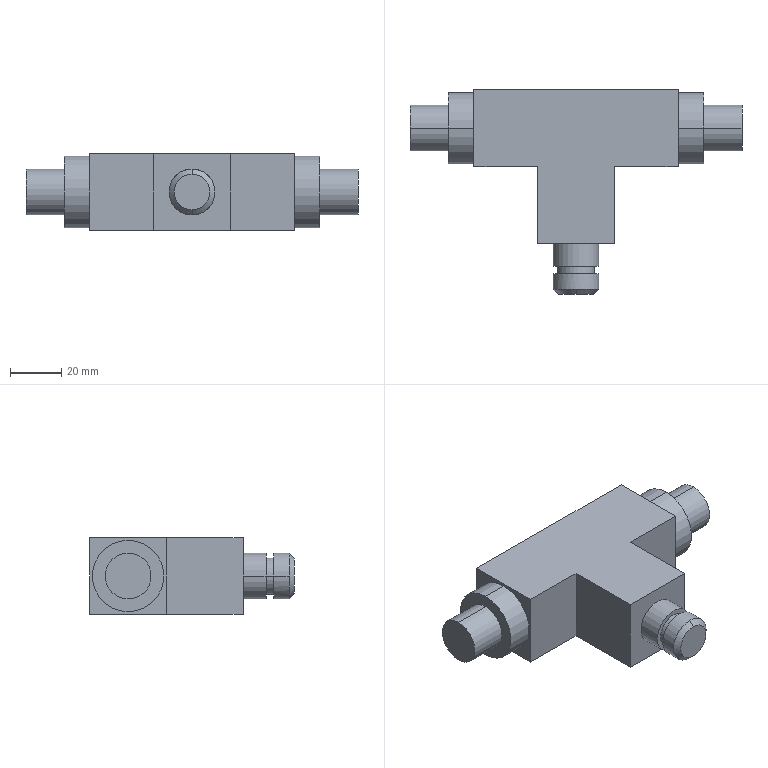Part | SolidWorks | features ICE 6, Chamfer 1, Cut 1, Extrusion 1 | 1 solid | 39 faces | box 130 x 80 x 30 mm | volume 123416 mm3 | plane 19 | cylinder 18 | cone 2 | commonest cylinder face diameters 18 x8 5 x4 28 x4 14.296 x2
STEP:
#1=CARTESIAN_POINT('',(-17.5,45.,6.));
#2=VERTEX_POINT('',#1);
#3=CARTESIAN_POINT('',(-22.5,45.,6.));
#4=VERTEX_POINT('',#3);
#5=CARTESIAN_POINT('',(-20.,45.,6.));
#6=DIRECTION('',(0.,0.,-1.));
#7=DIRECTION('',(-1.,0.,0.));
#8=AXIS2_PLACEMENT_3D('',#5,#6,#7);
#9=CIRCLE('',#8,2.5);
#10=EDGE_CURVE('',#2,#4,#9,.T.);
#11=ORIENTED_EDGE('',*,*,#10,.F.);
#12=CARTESIAN_POINT('',(-17.5,45.,0.));
#13=VERTEX_POINT('',#12);
#14=CARTESIAN_POINT('',(-17.5,45.,6.));
#15=DIRECTION('',(0.,0.,-1.));
#16=VECTOR('',#15,1000.);
#17=LINE('',#14,#16);
#18=EDGE_CURVE('',#2,#13,#17,.T.);
#19=ORIENTED_EDGE('',*,*,#18,.T.);
#20=CARTESIAN_POINT('',(-22.5,45.,0.));
#21=VERTEX_POINT('',#20);
#22=CARTESIAN_POINT('',(-20.,45.,0.));
#23=DIRECTION('',(0.,0.,-1.));
#24=DIRECTION('',(-1.,0.,0.));
#25=AXIS2_PLACEMENT_3D('',#22,#23,#24);
#26=CIRCLE('',#25,2.5);
#27=EDGE_CURVE('',#13,#21,#26,.T.);
#28=ORIENTED_EDGE('',*,*,#27,.T.);
#29=CARTESIAN_POINT('',(-22.5,45.,6.));
#30=DIRECTION('',(0.,0.,-1.));
#31=VECTOR('',#30,1000.);
#32=LINE('',#29,#31);
#33=EDGE_CURVE('',#4,#21,#32,.T.);
#34=ORIENTED_EDGE('',*,*,#33,.F.);
#35=EDGE_LOOP('',(#11,#19,#28,#34));
#36=FACE_OUTER_BOUND('',#35,.T.);
#37=CARTESIAN_POINT('',(-20.,45.,6.));
#38=DIRECTION('',(0.,0.,-1.));
#39=DIRECTION('',(-1.,0.,0.));
#40=AXIS2_PLACEMENT_3D('',#37,#38,#39);
#41=CYLINDRICAL_SURFACE('',#40,2.5);
#42=ADVANCED_FACE('',(#36),#41,.F.);
#43=CARTESIAN_POINT('',(52.5,45.,6.));
#44=VERTEX_POINT('',#43);
#45=CARTESIAN_POINT('',(47.5,45.,6.));
#46=VERTEX_POINT('',#45);
#47=CARTESIAN_POINT('',(50.,45.,6.));
#48=DIRECTION('',(0.,0.,-1.));
#49=DIRECTION('',(-1.,0.,0.));
#50=AXIS2_PLACEMENT_3D('',#47,#48,#49);
#51=CIRCLE('',#50,2.5);
#52=EDGE_CURVE('',#44,#46,#51,.T.);
#53=ORIENTED_EDGE('',*,*,#52,.F.);
#54=CARTESIAN_POINT('',(52.5,45.,0.));
#55=VERTEX_POINT('',#54);
#56=CARTESIAN_POINT('',(52.5,45.,6.));
#57=DIRECTION('',(0.,0.,-1.));
#58=VECTOR('',#57,1000.);
#59=LINE('',#56,#58);
#60=EDGE_CURVE('',#44,#55,#59,.T.);
#61=ORIENTED_EDGE('',*,*,#60,.T.);
#62=CARTESIAN_POINT('',(47.5,45.,0.));
#63=VERTEX_POINT('',#62);
#64=CARTESIAN_POINT('',(50.,45.,0.));
#65=DIRECTION('',(0.,0.,-1.));
#66=DIRECTION('',(-1.,0.,0.));
#67=AXIS2_PLACEMENT_3D('',#64,#65,#66);
#68=CIRCLE('',#67,2.5);
#69=EDGE_CURVE('',#55,#63,#68,.T.);
#70=ORIENTED_EDGE('',*,*,#69,.T.);
#71=CARTESIAN_POINT('',(47.5,45.,6.));
#72=DIRECTION('',(0.,0.,-1.));
#73=VECTOR('',#72,1000.);
#74=LINE('',#71,#73);
#75=EDGE_CURVE('',#46,#63,#74,.T.);
#76=ORIENTED_EDGE('',*,*,#75,.F.);
#77=EDGE_LOOP('',(#53,#61,#70,#76));
#78=FACE_OUTER_BOUND('',#77,.T.);
#79=CARTESIAN_POINT('',(50.,45.,6.));
#80=DIRECTION('',(0.,0.,-1.));
#81=DIRECTION('',(-1.,0.,0.));
#82=AXIS2_PLACEMENT_3D('',#79,#80,#81);
#83=CYLINDRICAL_SURFACE('',#82,2.5);
#84=ADVANCED_FACE('',(#78),#83,.F.);
#85=CARTESIAN_POINT('',(15.,-20.,8.));
#86=VERTEX_POINT('',#85);
#87=CARTESIAN_POINT('',(15.,-20.,22.));
#88=VERTEX_POINT('',#87);
#89=CARTESIAN_POINT('',(15.,-20.,15.));
#90=DIRECTION('',(0.,-1.,0.));
#91=DIRECTION('',(1.,0.,0.));
#92=AXIS2_PLACEMENT_3D('',#89,#90,#91);
#93=CIRCLE('',#92,7.);
#94=EDGE_CURVE('',#86,#88,#93,.T.);
#95=ORIENTED_EDGE('',*,*,#94,.F.);
#96=CARTESIAN_POINT('',(15.,-18.,6.));
#97=VERTEX_POINT('',#96);
#98=CARTESIAN_POINT('',(15.,-20.,8.));
#99=DIRECTION('',(0.,0.7071,-0.7071));
#100=VECTOR('',#99,1000.);
#101=LINE('',#98,#100);
#102=EDGE_CURVE('',#86,#97,#101,.T.);
#103=ORIENTED_EDGE('',*,*,#102,.T.);
#104=CARTESIAN_POINT('',(24.,-18.,15.));
#105=VERTEX_POINT('',#104);
#106=CARTESIAN_POINT('',(15.,-18.,15.));
#107=DIRECTION('',(0.,1.,0.));
#108=DIRECTION('',(0.,0.,-1.));
#109=AXIS2_PLACEMENT_3D('',#106,#107,#108);
#110=CIRCLE('',#109,9.);
#111=EDGE_CURVE('',#105,#97,#110,.T.);
#112=ORIENTED_EDGE('',*,*,#111,.F.);
#113=CARTESIAN_POINT('',(15.,-18.,24.));
#114=VERTEX_POINT('',#113);
#115=CARTESIAN_POINT('',(15.,-18.,15.));
#116=DIRECTION('',(0.,1.,0.));
#117=DIRECTION('',(0.,0.,-1.));
#118=AXIS2_PLACEMENT_3D('',#115,#116,#117);
#119=CIRCLE('',#118,9.);
#120=EDGE_CURVE('',#114,#105,#119,.T.);
#121=ORIENTED_EDGE('',*,*,#120,.F.);
#122=CARTESIAN_POINT('',(15.,-20.,22.));
#123=DIRECTION('',(0.,0.7071,0.7071));
#124=VECTOR('',#123,1000.);
#125=LINE('',#122,#124);
#126=EDGE_CURVE('',#88,#114,#125,.T.);
#127=ORIENTED_EDGE('',*,*,#126,.F.);
#128=EDGE_LOOP('',(#95,#103,#112,#121,#127));
#129=FACE_OUTER_BOUND('',#128,.T.);
#130=CARTESIAN_POINT('',(15.,-20.,15.));
#131=DIRECTION('',(0.,1.,0.));
#132=DIRECTION('',(0.,0.,1.));
#133=AXIS2_PLACEMENT_3D('',#130,#131,#132);
#134=CONICAL_SURFACE('',#133,7.,0.7854);
#135=ADVANCED_FACE('',(#129),#134,.T.);
#136=CARTESIAN_POINT('',(6.,-18.,15.));
#137=VERTEX_POINT('',#136);
#138=CARTESIAN_POINT('',(15.,-18.,15.));
#139=DIRECTION('',(0.,1.,0.));
#140=DIRECTION('',(0.,0.,-1.));
#141=AXIS2_PLACEMENT_3D('',#138,#139,#140);
#142=CIRCLE('',#141,9.);
#143=EDGE_CURVE('',#137,#114,#142,.T.);
#144=ORIENTED_EDGE('',*,*,#143,.T.);
#145=ORIENTED_EDGE('',*,*,#120,.T.);
#146=CARTESIAN_POINT('',(24.,-12.,15.));
#147=VERTEX_POINT('',#146);
#148=CARTESIAN_POINT('',(24.,-20.,15.));
#149=DIRECTION('',(0.,1.,0.));
#150=VECTOR('',#149,1000.);
#151=LINE('',#148,#150);
#152=EDGE_CURVE('',#105,#147,#151,.T.);
#153=ORIENTED_EDGE('',*,*,#152,.T.);
#154=CARTESIAN_POINT('',(6.,-12.,15.));
#155=VERTEX_POINT('',#154);
#156=CARTESIAN_POINT('',(15.,-12.,15.));
#157=DIRECTION('',(0.,-1.,0.));
#158=DIRECTION('',(1.,0.,0.));
#159=AXIS2_PLACEMENT_3D('',#156,#157,#158);
#160=CIRCLE('',#159,9.);
#161=EDGE_CURVE('',#147,#155,#160,.T.);
#162=ORIENTED_EDGE('',*,*,#161,.T.);
#163=CARTESIAN_POINT('',(6.,-20.,15.));
#164=DIRECTION('',(0.,1.,0.));
#165=VECTOR('',#164,1000.);
#166=LINE('',#163,#165);
#167=EDGE_CURVE('',#137,#155,#166,.T.);
#168=ORIENTED_EDGE('',*,*,#167,.F.);
#169=EDGE_LOOP('',(#144,#145,#153,#162,#168));
#170=FACE_OUTER_BOUND('',#169,.T.);
#171=CARTESIAN_POINT('',(15.,-20.,15.));
#172=DIRECTION('',(0.,1.,0.));
#173=DIRECTION('',(-1.,0.,0.));
#174=AXIS2_PLACEMENT_3D('',#171,#172,#173);
#175=CYLINDRICAL_SURFACE('',#174,9.);
#176=ADVANCED_FACE('',(#170),#175,.T.);
#177=CARTESIAN_POINT('',(22.148,-9.,15.));
#178=VERTEX_POINT('',#177);
#179=CARTESIAN_POINT('',(7.852,-9.,15.));
#180=VERTEX_POINT('',#179);
#181=CARTESIAN_POINT('',(15.,-9.,15.));
#182=DIRECTION('',(0.,-1.,0.));
#183=DIRECTION('',(1.,0.,0.));
#184=AXIS2_PLACEMENT_3D('',#181,#182,#183);
#185=CIRCLE('',#184,7.148);
#186=EDGE_CURVE('',#178,#180,#185,.T.);
#187=ORIENTED_EDGE('',*,*,#186,.T.);
#188=CARTESIAN_POINT('',(7.852,-12.,15.));
#189=VERTEX_POINT('',#188);
#190=CARTESIAN_POINT('',(7.852,-9.,15.));
#191=DIRECTION('',(0.,-1.,0.));
#192=VECTOR('',#191,1000.);
#193=LINE('',#190,#192);
#194=EDGE_CURVE('',#180,#189,#193,.T.);
#195=ORIENTED_EDGE('',*,*,#194,.T.);
#196=CARTESIAN_POINT('',(22.148,-12.,15.));
#197=VERTEX_POINT('',#196);
#198=CARTESIAN_POINT('',(15.,-12.,15.));
#199=DIRECTION('',(0.,-1.,0.));
#200=DIRECTION('',(1.,0.,0.));
#201=AXIS2_PLACEMENT_3D('',#198,#199,#200);
#202=CIRCLE('',#201,7.148);
#203=EDGE_CURVE('',#197,#189,#202,.T.);
#204=ORIENTED_EDGE('',*,*,#203,.F.);
#205=CARTESIAN_POINT('',(22.148,-9.,15.));
#206=DIRECTION('',(0.,-1.,0.));
#207=VECTOR('',#206,1000.);
#208=LINE('',#205,#207);
#209=EDGE_CURVE('',#178,#197,#208,.T.);
#210=ORIENTED_EDGE('',*,*,#209,.F.);
#211=EDGE_LOOP('',(#187,#195,#204,#210));
#212=FACE_OUTER_BOUND('',#211,.T.);
#213=CARTESIAN_POINT('',(15.,-9.,15.));
#214=DIRECTION('',(0.,-1.,0.));
#215=DIRECTION('',(1.,0.,0.));
#216=AXIS2_PLACEMENT_3D('',#213,#214,#215);
#217=CYLINDRICAL_SURFACE('',#216,7.148);
#218=ADVANCED_FACE('',(#212),#217,.T.);
#219=CARTESIAN_POINT('',(-50.,45.,24.));
#220=VERTEX_POINT('',#219);
#221=CARTESIAN_POINT('',(-50.,45.,6.));
#222=VERTEX_POINT('',#221);
#223=CARTESIAN_POINT('',(-50.,45.,15.));
#224=DIRECTION('',(-1.,0.,0.));
#225=DIRECTION('',(0.,0.,1.));
#226=AXIS2_PLACEMENT_3D('',#223,#224,#225);
#227=CIRCLE('',#226,9.);
#228=EDGE_CURVE('',#220,#222,#227,.T.);
#229=ORIENTED_EDGE('',*,*,#228,.F.);
#230=CARTESIAN_POINT('',(-35.,45.,24.));
#231=VERTEX_POINT('',#230);
#232=CARTESIAN_POINT('',(-50.,45.,24.));
#233=DIRECTION('',(1.,0.,0.));
#234=VECTOR('',#233,1000.);
#235=LINE('',#232,#234);
#236=EDGE_CURVE('',#220,#231,#235,.T.);
#237=ORIENTED_EDGE('',*,*,#236,.T.);
#238=CARTESIAN_POINT('',(-35.,45.,6.));
#239=VERTEX_POINT('',#238);
#240=CARTESIAN_POINT('',(-35.,45.,15.));
#241=DIRECTION('',(-1.,0.,0.));
#242=DIRECTION('',(0.,0.,1.));
#243=AXIS2_PLACEMENT_3D('',#240,#241,#242);
#244=CIRCLE('',#243,9.);
#245=EDGE_CURVE('',#231,#239,#244,.T.);
#246=ORIENTED_EDGE('',*,*,#245,.T.);
#247=CARTESIAN_POINT('',(-50.,45.,6.));
#248=DIRECTION('',(1.,0.,0.));
#249=VECTOR('',#248,1000.);
#250=LINE('',#247,#249);
#251=EDGE_CURVE('',#222,#239,#250,.T.);
#252=ORIENTED_EDGE('',*,*,#251,.F.);
#253=EDGE_LOOP('',(#229,#237,#246,#252));
#254=FACE_OUTER_BOUND('',#253,.T.);
#255=CARTESIAN_POINT('',(-50.,45.,15.));
#256=DIRECTION('',(1.,0.,0.));
#257=DIRECTION('',(0.,0.,-1.));
#258=AXIS2_PLACEMENT_3D('',#255,#256,#257);
#259=CYLINDRICAL_SURFACE('',#258,9.);
#260=ADVANCED_FACE('',(#254),#259,.T.);
#261=CARTESIAN_POINT('',(-35.,45.,29.));
#262=VERTEX_POINT('',#261);
#263=CARTESIAN_POINT('',(-35.,45.,1.));
#264=VERTEX_POINT('',#263);
#265=CARTESIAN_POINT('',(-35.,45.,15.));
#266=DIRECTION('',(-1.,0.,0.));
#267=DIRECTION('',(0.,0.,1.));
#268=AXIS2_PLACEMENT_3D('',#265,#266,#267);
#269=CIRCLE('',#268,14.);
#270=EDGE_CURVE('',#262,#264,#269,.T.);
#271=ORIENTED_EDGE('',*,*,#270,.F.);
#272=CARTESIAN_POINT('',(-25.,45.,29.));
#273=VERTEX_POINT('',#272);
#274=CARTESIAN_POINT('',(-35.,45.,29.));
#275=DIRECTION('',(1.,0.,0.));
#276=VECTOR('',#275,1000.);
#277=LINE('',#274,#276);
#278=EDGE_CURVE('',#262,#273,#277,.T.);
#279=ORIENTED_EDGE('',*,*,#278,.T.);
#280=CARTESIAN_POINT('',(-25.,45.,1.));
#281=VERTEX_POINT('',#280);
#282=CARTESIAN_POINT('',(-25.,45.,15.));
#283=DIRECTION('',(-1.,0.,0.));
#284=DIRECTION('',(0.,0.,-1.));
#285=AXIS2_PLACEMENT_3D('',#282,#283,#284);
#286=CIRCLE('',#285,14.);
#287=EDGE_CURVE('',#273,#281,#286,.T.);
#288=ORIENTED_EDGE('',*,*,#287,.T.);
#289=CARTESIAN_POINT('',(-35.,45.,1.));
#290=DIRECTION('',(1.,0.,0.));
#291=VECTOR('',#290,1000.);
#292=LINE('',#289,#291);
#293=EDGE_CURVE('',#264,#281,#292,.T.);
#294=ORIENTED_EDGE('',*,*,#293,.F.);
#295=EDGE_LOOP('',(#271,#279,#288,#294));
#296=FACE_OUTER_BOUND('',#295,.T.);
#297=CARTESIAN_POINT('',(-35.,45.,15.));
#298=DIRECTION('',(1.,0.,0.));
#299=DIRECTION('',(0.,0.,-1.));
#300=AXIS2_PLACEMENT_3D('',#297,#298,#299);
#301=CYLINDRICAL_SURFACE('',#300,14.);
#302=ADVANCED_FACE('',(#296),#301,.T.);
#303=CARTESIAN_POINT('',(80.,45.,6.));
#304=VERTEX_POINT('',#303);
#305=CARTESIAN_POINT('',(80.,45.,24.));
#306=VERTEX_POINT('',#305);
#307=CARTESIAN_POINT('',(80.,45.,15.));
#308=DIRECTION('',(1.,0.,0.));
#309=DIRECTION('',(0.,0.,-1.));
#310=AXIS2_PLACEMENT_3D('',#307,#308,#309);
#311=CIRCLE('',#310,9.);
#312=EDGE_CURVE('',#304,#306,#311,.T.);
#313=ORIENTED_EDGE('',*,*,#312,.F.);
#314=CARTESIAN_POINT('',(65.,45.,6.));
#315=VERTEX_POINT('',#314);
#316=CARTESIAN_POINT('',(80.,45.,6.));
#317=DIRECTION('',(-1.,0.,0.));
#318=VECTOR('',#317,1000.);
#319=LINE('',#316,#318);
#320=EDGE_CURVE('',#304,#315,#319,.T.);
#321=ORIENTED_EDGE('',*,*,#320,.T.);
#322=CARTESIAN_POINT('',(65.,45.,24.));
#323=VERTEX_POINT('',#322);
#324=CARTESIAN_POINT('',(65.,45.,15.));
#325=DIRECTION('',(1.,0.,0.));
#326=DIRECTION('',(0.,0.,-1.));
#327=AXIS2_PLACEMENT_3D('',#324,#325,#326);
#328=CIRCLE('',#327,9.);
#329=EDGE_CURVE('',#315,#323,#328,.T.);
#330=ORIENTED_EDGE('',*,*,#329,.T.);
#331=CARTESIAN_POINT('',(80.,45.,24.));
#332=DIRECTION('',(-1.,0.,0.));
#333=VECTOR('',#332,1000.);
#334=LINE('',#331,#333);
#335=EDGE_CURVE('',#306,#323,#334,.T.);
#336=ORIENTED_EDGE('',*,*,#335,.F.);
#337=EDGE_LOOP('',(#313,#321,#330,#336));
#338=FACE_OUTER_BOUND('',#337,.T.);
#339=CARTESIAN_POINT('',(80.,45.,15.));
#340=DIRECTION('',(-1.,0.,0.));
#341=DIRECTION('',(0.,0.,1.));
#342=AXIS2_PLACEMENT_3D('',#339,#340,#341);
#343=CYLINDRICAL_SURFACE('',#342,9.);
#344=ADVANCED_FACE('',(#338),#343,.T.);
#345=CARTESIAN_POINT('',(65.,45.,1.));
#346=VERTEX_POINT('',#345);
#347=CARTESIAN_POINT('',(65.,45.,29.));
#348=VERTEX_POINT('',#347);
#349=CARTESIAN_POINT('',(65.,45.,15.));
#350=DIRECTION('',(1.,0.,0.));
#351=DIRECTION('',(0.,0.,-1.));
#352=AXIS2_PLACEMENT_3D('',#349,#350,#351);
#353=CIRCLE('',#352,14.);
#354=EDGE_CURVE('',#346,#348,#353,.T.);
#355=ORIENTED_EDGE('',*,*,#354,.F.);
#356=CARTESIAN_POINT('',(55.,45.,1.));
#357=VERTEX_POINT('',#356);
#358=CARTESIAN_POINT('',(65.,45.,1.));
#359=DIRECTION('',(-1.,0.,0.));
#360=VECTOR('',#359,1000.);
#361=LINE('',#358,#360);
#362=EDGE_CURVE('',#346,#357,#361,.T.);
#363=ORIENTED_EDGE('',*,*,#362,.T.);
#364=CARTESIAN_POINT('',(55.,45.,29.));
#365=VERTEX_POINT('',#364);
#366=CARTESIAN_POINT('',(55.,45.,15.));
#367=DIRECTION('',(1.,0.,0.));
#368=DIRECTION('',(0.,-1.,0.));
#369=AXIS2_PLACEMENT_3D('',#366,#367,#368);
#370=CIRCLE('',#369,14.);
#371=EDGE_CURVE('',#357,#365,#370,.T.);
#372=ORIENTED_EDGE('',*,*,#371,.T.);
#373=CARTESIAN_POINT('',(65.,45.,29.));
#374=DIRECTION('',(-1.,0.,0.));
#375=VECTOR('',#374,1000.);
#376=LINE('',#373,#375);
#377=EDGE_CURVE('',#348,#365,#376,.T.);
#378=ORIENTED_EDGE('',*,*,#377,.F.);
#379=EDGE_LOOP('',(#355,#363,#372,#378));
#380=FACE_OUTER_BOUND('',#379,.T.);
#381=CARTESIAN_POINT('',(65.,45.,15.));
#382=DIRECTION('',(-1.,0.,0.));
#383=DIRECTION('',(0.,0.,1.));
#384=AXIS2_PLACEMENT_3D('',#381,#382,#383);
#385=CYLINDRICAL_SURFACE('',#384,14.);
#386=ADVANCED_FACE('',(#380),#385,.T.);
#387=CARTESIAN_POINT('',(24.,-9.,15.));
#388=VERTEX_POINT('',#387);
#389=CARTESIAN_POINT('',(6.,-9.,15.));
#390=VERTEX_POINT('',#389);
#391=CARTESIAN_POINT('',(15.,-9.,15.));
#392=DIRECTION('',(0.,-1.,0.));
#393=DIRECTION('',(1.,0.,0.));
#394=AXIS2_PLACEMENT_3D('',#391,#392,#393);
#395=CIRCLE('',#394,9.);
#396=EDGE_CURVE('',#388,#390,#395,.T.);
#397=ORIENTED_EDGE('',*,*,#396,.F.);
#398=CARTESIAN_POINT('',(24.,0.,15.));
#399=VERTEX_POINT('',#398);
#400=CARTESIAN_POINT('',(24.,-20.,15.));
#401=DIRECTION('',(0.,1.,0.));
#402=VECTOR('',#401,1000.);
#403=LINE('',#400,#402);
#404=EDGE_CURVE('',#388,#399,#403,.T.);
#405=ORIENTED_EDGE('',*,*,#404,.T.);
#406=CARTESIAN_POINT('',(6.,0.,15.));
#407=VERTEX_POINT('',#406);
#408=CARTESIAN_POINT('',(15.,0.,15.));
#409=DIRECTION('',(0.,-1.,0.));
#410=DIRECTION('',(-1.,0.,0.));
#411=AXIS2_PLACEMENT_3D('',#408,#409,#410);
#412=CIRCLE('',#411,9.);
#413=EDGE_CURVE('',#399,#407,#412,.T.);
#414=ORIENTED_EDGE('',*,*,#413,.T.);
#415=CARTESIAN_POINT('',(6.,-20.,15.));
#416=DIRECTION('',(0.,1.,0.));
#417=VECTOR('',#416,1000.);
#418=LINE('',#415,#417);
#419=EDGE_CURVE('',#390,#407,#418,.T.);
#420=ORIENTED_EDGE('',*,*,#419,.F.);
#421=EDGE_LOOP('',(#397,#405,#414,#420));
#422=FACE_OUTER_BOUND('',#421,.T.);
#423=CARTESIAN_POINT('',(15.,-20.,15.));
#424=DIRECTION('',(0.,1.,0.));
#425=DIRECTION('',(-1.,0.,0.));
#426=AXIS2_PLACEMENT_3D('',#423,#424,#425);
#427=CYLINDRICAL_SURFACE('',#426,9.);
#428=ADVANCED_FACE('',(#422),#427,.T.);
#429=ORIENTED_EDGE('',*,*,#404,.F.);
#430=CARTESIAN_POINT('',(15.,-9.,15.));
#431=DIRECTION('',(0.,-1.,0.));
#432=DIRECTION('',(1.,0.,0.));
#433=AXIS2_PLACEMENT_3D('',#430,#431,#432);
#434=CIRCLE('',#433,9.);
#435=EDGE_CURVE('',#390,#388,#434,.T.);
#436=ORIENTED_EDGE('',*,*,#435,.F.);
#437=ORIENTED_EDGE('',*,*,#419,.T.);
#438=CARTESIAN_POINT('',(15.,0.,15.));
#439=DIRECTION('',(0.,-1.,0.));
#440=DIRECTION('',(-1.,0.,0.));
#441=AXIS2_PLACEMENT_3D('',#438,#439,#440);
#442=CIRCLE('',#441,9.);
#443=EDGE_CURVE('',#407,#399,#442,.T.);
#444=ORIENTED_EDGE('',*,*,#443,.T.);
#445=EDGE_LOOP('',(#429,#436,#437,#444));
#446=FACE_OUTER_BOUND('',#445,.T.);
#447=CARTESIAN_POINT('',(15.,-20.,15.));
#448=DIRECTION('',(0.,1.,0.));
#449=DIRECTION('',(-1.,0.,0.));
#450=AXIS2_PLACEMENT_3D('',#447,#448,#449);
#451=CYLINDRICAL_SURFACE('',#450,9.);
#452=ADVANCED_FACE('',(#446),#451,.T.);
#453=ORIENTED_EDGE('',*,*,#443,.F.);
#454=ORIENTED_EDGE('',*,*,#413,.F.);
#455=EDGE_LOOP('',(#453,#454));
#456=FACE_BOUND('',#455,.T.);
#457=CARTESIAN_POINT('',(0.,0.,0.));
#458=VERTEX_POINT('',#457);
#459=CARTESIAN_POINT('',(30.,0.,0.));
#460=VERTEX_POINT('',#459);
#461=CARTESIAN_POINT('',(30.,0.,0.));
#462=DIRECTION('',(1.,0.,0.));
#463=VECTOR('',#462,1000.);
#464=LINE('',#461,#463);
#465=EDGE_CURVE('',#458,#460,#464,.T.);
#466=ORIENTED_EDGE('',*,*,#465,.T.);
#467=CARTESIAN_POINT('',(30.,0.,30.));
#468=VERTEX_POINT('',#467);
#469=CARTESIAN_POINT('',(30.,0.,30.));
#470=DIRECTION('',(0.,0.,-1.));
#471=VECTOR('',#470,1000.);
#472=LINE('',#469,#471);
#473=EDGE_CURVE('',#468,#460,#472,.T.);
#474=ORIENTED_EDGE('',*,*,#473,.F.);
#475=CARTESIAN_POINT('',(0.,0.,30.));
#476=VERTEX_POINT('',#475);
#477=CARTESIAN_POINT('',(30.,0.,30.));
#478=DIRECTION('',(1.,0.,0.));
#479=VECTOR('',#478,1000.);
#480=LINE('',#477,#479);
#481=EDGE_CURVE('',#476,#468,#480,.T.);
#482=ORIENTED_EDGE('',*,*,#481,.F.);
#483=CARTESIAN_POINT('',(0.,0.,30.));
#484=DIRECTION('',(0.,0.,-1.));
#485=VECTOR('',#484,1000.);
#486=LINE('',#483,#485);
#487=EDGE_CURVE('',#476,#458,#486,.T.);
#488=ORIENTED_EDGE('',*,*,#487,.T.);
#489=EDGE_LOOP('',(#466,#474,#482,#488));
#490=FACE_OUTER_BOUND('',#489,.T.);
#491=CARTESIAN_POINT('',(30.,0.,30.));
#492=DIRECTION('',(0.,1.,0.));
#493=DIRECTION('',(-1.,0.,0.));
#494=AXIS2_PLACEMENT_3D('',#491,#492,#493);
#495=PLANE('',#494);
#496=ADVANCED_FACE('',(#456,#490),#495,.F.);
#497=CARTESIAN_POINT('',(30.,30.,0.));
#498=VERTEX_POINT('',#497);
#499=CARTESIAN_POINT('',(30.,30.,0.));
#500=DIRECTION('',(0.,1.,0.));
#501=VECTOR('',#500,1000.);
#502=LINE('',#499,#501);
#503=EDGE_CURVE('',#460,#498,#502,.T.);
#504=ORIENTED_EDGE('',*,*,#503,.T.);
#505=CARTESIAN_POINT('',(30.,30.,30.));
#506=VERTEX_POINT('',#505);
#507=CARTESIAN_POINT('',(30.,30.,30.));
#508=DIRECTION('',(0.,0.,-1.));
#509=VECTOR('',#508,1000.);
#510=LINE('',#507,#509);
#511=EDGE_CURVE('',#506,#498,#510,.T.);
#512=ORIENTED_EDGE('',*,*,#511,.F.);
#513=CARTESIAN_POINT('',(30.,30.,30.));
#514=DIRECTION('',(0.,1.,0.));
#515=VECTOR('',#514,1000.);
#516=LINE('',#513,#515);
#517=EDGE_CURVE('',#468,#506,#516,.T.);
#518=ORIENTED_EDGE('',*,*,#517,.F.);
#519=ORIENTED_EDGE('',*,*,#473,.T.);
#520=EDGE_LOOP('',(#504,#512,#518,#519));
#521=FACE_OUTER_BOUND('',#520,.T.);
#522=CARTESIAN_POINT('',(30.,30.,30.));
#523=DIRECTION('',(-1.,0.,0.));
#524=DIRECTION('',(0.,-1.,0.));
#525=AXIS2_PLACEMENT_3D('',#522,#523,#524);
#526=PLANE('',#525);
#527=ADVANCED_FACE('',(#521),#526,.F.);
#528=CARTESIAN_POINT('',(55.,30.,0.));
#529=VERTEX_POINT('',#528);
#530=CARTESIAN_POINT('',(55.,30.,0.));
#531=DIRECTION('',(1.,0.,0.));
#532=VECTOR('',#531,1000.);
#533=LINE('',#530,#532);
#534=EDGE_CURVE('',#498,#529,#533,.T.);
#535=ORIENTED_EDGE('',*,*,#534,.T.);
#536=CARTESIAN_POINT('',(55.,30.,30.));
#537=VERTEX_POINT('',#536);
#538=CARTESIAN_POINT('',(55.,30.,30.));
#539=DIRECTION('',(0.,0.,-1.));
#540=VECTOR('',#539,1000.);
#541=LINE('',#538,#540);
#542=EDGE_CURVE('',#537,#529,#541,.T.);
#543=ORIENTED_EDGE('',*,*,#542,.F.);
#544=CARTESIAN_POINT('',(55.,30.,30.));
#545=DIRECTION('',(1.,0.,0.));
#546=VECTOR('',#545,1000.);
#547=LINE('',#544,#546);
#548=EDGE_CURVE('',#506,#537,#547,.T.);
#549=ORIENTED_EDGE('',*,*,#548,.F.);
#550=ORIENTED_EDGE('',*,*,#511,.T.);
#551=EDGE_LOOP('',(#535,#543,#549,#550));
#552=FACE_OUTER_BOUND('',#551,.T.);
#553=CARTESIAN_POINT('',(55.,30.,30.));
#554=DIRECTION('',(0.,1.,0.));
#555=DIRECTION('',(0.,0.,1.));
#556=AXIS2_PLACEMENT_3D('',#553,#554,#555);
#557=PLANE('',#556);
#558=ADVANCED_FACE('',(#552),#557,.F.);
#559=CARTESIAN_POINT('',(55.,45.,15.));
#560=DIRECTION('',(1.,0.,0.));
#561=DIRECTION('',(0.,-1.,0.));
#562=AXIS2_PLACEMENT_3D('',#559,#560,#561);
#563=CIRCLE('',#562,14.);
#564=EDGE_CURVE('',#365,#357,#563,.T.);
#565=ORIENTED_EDGE('',*,*,#564,.F.);
#566=ORIENTED_EDGE('',*,*,#371,.F.);
#567=EDGE_LOOP('',(#565,#566));
#568=FACE_BOUND('',#567,.T.);
#569=CARTESIAN_POINT('',(55.,60.,0.));
#570=VERTEX_POINT('',#569);
#571=CARTESIAN_POINT('',(55.,60.,0.));
#572=DIRECTION('',(0.,1.,0.));
#573=VECTOR('',#572,1000.);
#574=LINE('',#571,#573);
#575=EDGE_CURVE('',#529,#570,#574,.T.);
#576=ORIENTED_EDGE('',*,*,#575,.T.);
#577=CARTESIAN_POINT('',(55.,60.,30.));
#578=VERTEX_POINT('',#577);
#579=CARTESIAN_POINT('',(55.,60.,30.));
#580=DIRECTION('',(0.,0.,-1.));
#581=VECTOR('',#580,1000.);
#582=LINE('',#579,#581);
#583=EDGE_CURVE('',#578,#570,#582,.T.);
#584=ORIENTED_EDGE('',*,*,#583,.F.);
#585=CARTESIAN_POINT('',(55.,60.,30.));
#586=DIRECTION('',(0.,1.,0.));
#587=VECTOR('',#586,1000.);
#588=LINE('',#585,#587);
#589=EDGE_CURVE('',#537,#578,#588,.T.);
#590=ORIENTED_EDGE('',*,*,#589,.F.);
#591=ORIENTED_EDGE('',*,*,#542,.T.);
#592=EDGE_LOOP('',(#576,#584,#590,#591));
#593=FACE_OUTER_BOUND('',#592,.T.);
#594=CARTESIAN_POINT('',(55.,60.,30.));
#595=DIRECTION('',(-1.,0.,0.));
#596=DIRECTION('',(0.,-1.,0.));
#597=AXIS2_PLACEMENT_3D('',#594,#595,#596);
#598=PLANE('',#597);
#599=ADVANCED_FACE('',(#568,#593),#598,.F.);
#600=CARTESIAN_POINT('',(-25.,60.,0.));
#601=VERTEX_POINT('',#600);
#602=CARTESIAN_POINT('',(-25.,60.,0.));
#603=DIRECTION('',(-1.,0.,0.));
#604=VECTOR('',#603,1000.);
#605=LINE('',#602,#604);
#606=EDGE_CURVE('',#570,#601,#605,.T.);
#607=ORIENTED_EDGE('',*,*,#606,.T.);
#608=CARTESIAN_POINT('',(-25.,60.,30.));
#609=VERTEX_POINT('',#608);
#610=CARTESIAN_POINT('',(-25.,60.,30.));
#611=DIRECTION('',(0.,0.,-1.));
#612=VECTOR('',#611,1000.);
#613=LINE('',#610,#612);
#614=EDGE_CURVE('',#609,#601,#613,.T.);
#615=ORIENTED_EDGE('',*,*,#614,.F.);
#616=CARTESIAN_POINT('',(-25.,60.,30.));
#617=DIRECTION('',(-1.,0.,0.));
#618=VECTOR('',#617,1000.);
#619=LINE('',#616,#618);
#620=EDGE_CURVE('',#578,#609,#619,.T.);
#621=ORIENTED_EDGE('',*,*,#620,.F.);
#622=ORIENTED_EDGE('',*,*,#583,.T.);
#623=EDGE_LOOP('',(#607,#615,#621,#622));
#624=FACE_OUTER_BOUND('',#623,.T.);
#625=CARTESIAN_POINT('',(-25.,60.,30.));
#626=DIRECTION('',(0.,-1.,0.));
#627=DIRECTION('',(1.,0.,0.));
#628=AXIS2_PLACEMENT_3D('',#625,#626,#627);
#629=PLANE('',#628);
#630=ADVANCED_FACE('',(#624),#629,.F.);
#631=CARTESIAN_POINT('',(-25.,45.,15.));
#632=DIRECTION('',(-1.,0.,0.));
#633=DIRECTION('',(0.,0.,-1.));
#634=AXIS2_PLACEMENT_3D('',#631,#632,#633);
#635=CIRCLE('',#634,14.);
#636=EDGE_CURVE('',#281,#273,#635,.T.);
#637=ORIENTED_EDGE('',*,*,#636,.F.);
#638=ORIENTED_EDGE('',*,*,#287,.F.);
#639=EDGE_LOOP('',(#637,#638));
#640=FACE_BOUND('',#639,.T.);
#641=CARTESIAN_POINT('',(-25.,30.,0.));
#642=VERTEX_POINT('',#641);
#643=CARTESIAN_POINT('',(-25.,30.,0.));
#644=DIRECTION('',(0.,-1.,0.));
#645=VECTOR('',#644,1000.);
#646=LINE('',#643,#645);
#647=EDGE_CURVE('',#601,#642,#646,.T.);
#648=ORIENTED_EDGE('',*,*,#647,.T.);
#649=CARTESIAN_POINT('',(-25.,30.,30.));
#650=VERTEX_POINT('',#649);
#651=CARTESIAN_POINT('',(-25.,30.,30.));
#652=DIRECTION('',(0.,0.,-1.));
#653=VECTOR('',#652,1000.);
#654=LINE('',#651,#653);
#655=EDGE_CURVE('',#650,#642,#654,.T.);
#656=ORIENTED_EDGE('',*,*,#655,.F.);
#657=CARTESIAN_POINT('',(-25.,30.,30.));
#658=DIRECTION('',(0.,-1.,0.));
#659=VECTOR('',#658,1000.);
#660=LINE('',#657,#659);
#661=EDGE_CURVE('',#609,#650,#660,.T.);
#662=ORIENTED_EDGE('',*,*,#661,.F.);
#663=ORIENTED_EDGE('',*,*,#614,.T.);
#664=EDGE_LOOP('',(#648,#656,#662,#663));
#665=FACE_OUTER_BOUND('',#664,.T.);
#666=CARTESIAN_POINT('',(-25.,30.,30.));
#667=DIRECTION('',(1.,0.,0.));
#668=DIRECTION('',(0.,0.,-1.));
#669=AXIS2_PLACEMENT_3D('',#666,#667,#668);
#670=PLANE('',#669);
#671=ADVANCED_FACE('',(#640,#665),#670,.F.);
#672=CARTESIAN_POINT('',(0.,30.,0.));
#673=VERTEX_POINT('',#672);
#674=CARTESIAN_POINT('',(0.,30.,0.));
#675=DIRECTION('',(1.,0.,0.));
#676=VECTOR('',#675,1000.);
#677=LINE('',#674,#676);
#678=EDGE_CURVE('',#642,#673,#677,.T.);
#679=ORIENTED_EDGE('',*,*,#678,.T.);
#680=CARTESIAN_POINT('',(0.,30.,30.));
#681=VERTEX_POINT('',#680);
#682=CARTESIAN_POINT('',(0.,30.,30.));
#683=DIRECTION('',(0.,0.,-1.));
#684=VECTOR('',#683,1000.);
#685=LINE('',#682,#684);
#686=EDGE_CURVE('',#681,#673,#685,.T.);
#687=ORIENTED_EDGE('',*,*,#686,.F.);
#688=CARTESIAN_POINT('',(0.,30.,30.));
#689=DIRECTION('',(1.,0.,0.));
#690=VECTOR('',#689,1000.);
#691=LINE('',#688,#690);
#692=EDGE_CURVE('',#650,#681,#691,.T.);
#693=ORIENTED_EDGE('',*,*,#692,.F.);
#694=ORIENTED_EDGE('',*,*,#655,.T.);
#695=EDGE_LOOP('',(#679,#687,#693,#694));
#696=FACE_OUTER_BOUND('',#695,.T.);
#697=CARTESIAN_POINT('',(0.,30.,30.));
#698=DIRECTION('',(0.,1.,0.));
#699=DIRECTION('',(-1.,0.,0.));
#700=AXIS2_PLACEMENT_3D('',#697,#698,#699);
#701=PLANE('',#700);
#702=ADVANCED_FACE('',(#696),#701,.F.);
#703=CARTESIAN_POINT('',(0.,0.,0.));
#704=DIRECTION('',(0.,-1.,0.));
#705=VECTOR('',#704,1000.);
#706=LINE('',#703,#705);
#707=EDGE_CURVE('',#673,#458,#706,.T.);
#708=ORIENTED_EDGE('',*,*,#707,.T.);
#709=ORIENTED_EDGE('',*,*,#487,.F.);
#710=CARTESIAN_POINT('',(0.,0.,30.));
#711=DIRECTION('',(0.,-1.,0.));
#712=VECTOR('',#711,1000.);
#713=LINE('',#710,#712);
#714=EDGE_CURVE('',#681,#476,#713,.T.);
#715=ORIENTED_EDGE('',*,*,#714,.F.);
#716=ORIENTED_EDGE('',*,*,#686,.T.);
#717=EDGE_LOOP('',(#708,#709,#715,#716));
#718=FACE_OUTER_BOUND('',#717,.T.);
#719=CARTESIAN_POINT('',(0.,0.,30.));
#720=DIRECTION('',(1.,0.,0.));
#721=DIRECTION('',(0.,0.,-1.));
#722=AXIS2_PLACEMENT_3D('',#719,#720,#721);
#723=PLANE('',#722);
#724=ADVANCED_FACE('',(#718),#723,.F.);
#725=ORIENTED_EDGE('',*,*,#481,.T.);
#726=ORIENTED_EDGE('',*,*,#517,.T.);
#727=ORIENTED_EDGE('',*,*,#548,.T.);
#728=ORIENTED_EDGE('',*,*,#589,.T.);
#729=ORIENTED_EDGE('',*,*,#620,.T.);
#730=ORIENTED_EDGE('',*,*,#661,.T.);
#731=ORIENTED_EDGE('',*,*,#692,.T.);
#732=ORIENTED_EDGE('',*,*,#714,.T.);
#733=EDGE_LOOP('',(#725,#726,#727,#728,#729,#730,#731,#732));
#734=FACE_OUTER_BOUND('',#733,.T.);
#735=CARTESIAN_POINT('',(0.,0.,30.));
#736=DIRECTION('',(0.,0.,-1.));
#737=DIRECTION('',(-1.,0.,0.));
#738=AXIS2_PLACEMENT_3D('',#735,#736,#737);
#739=PLANE('',#738);
#740=ADVANCED_FACE('',(#734),#739,.F.);
#741=CARTESIAN_POINT('',(-20.,45.,0.));
#742=DIRECTION('',(0.,0.,-1.));
#743=DIRECTION('',(-1.,0.,0.));
#744=AXIS2_PLACEMENT_3D('',#741,#742,#743);
#745=CIRCLE('',#744,2.5);
#746=EDGE_CURVE('',#21,#13,#745,.T.);
#747=ORIENTED_EDGE('',*,*,#746,.F.);
#748=ORIENTED_EDGE('',*,*,#27,.F.);
#749=EDGE_LOOP('',(#747,#748));
#750=FACE_BOUND('',#749,.T.);
#751=CARTESIAN_POINT('',(50.,45.,0.));
#752=DIRECTION('',(0.,0.,-1.));
#753=DIRECTION('',(-1.,0.,0.));
#754=AXIS2_PLACEMENT_3D('',#751,#752,#753);
#755=CIRCLE('',#754,2.5);
#756=EDGE_CURVE('',#63,#55,#755,.T.);
#757=ORIENTED_EDGE('',*,*,#756,.F.);
#758=ORIENTED_EDGE('',*,*,#69,.F.);
#759=EDGE_LOOP('',(#757,#758));
#760=FACE_BOUND('',#759,.T.);
#761=ORIENTED_EDGE('',*,*,#465,.F.);
#762=ORIENTED_EDGE('',*,*,#707,.F.);
#763=ORIENTED_EDGE('',*,*,#678,.F.);
#764=ORIENTED_EDGE('',*,*,#647,.F.);
#765=ORIENTED_EDGE('',*,*,#606,.F.);
#766=ORIENTED_EDGE('',*,*,#575,.F.);
#767=ORIENTED_EDGE('',*,*,#534,.F.);
#768=ORIENTED_EDGE('',*,*,#503,.F.);
#769=EDGE_LOOP('',(#761,#762,#763,#764,#765,#766,#767,#768));
#770=FACE_OUTER_BOUND('',#769,.T.);
#771=CARTESIAN_POINT('',(0.,0.,0.));
#772=DIRECTION('',(0.,0.,-1.));
#773=DIRECTION('',(-1.,0.,0.));
#774=AXIS2_PLACEMENT_3D('',#771,#772,#773);
#775=PLANE('',#774);
#776=ADVANCED_FACE('',(#750,#760,#770),#775,.T.);
#777=ORIENTED_EDGE('',*,*,#362,.F.);
#778=CARTESIAN_POINT('',(65.,45.,15.));
#779=DIRECTION('',(1.,0.,0.));
#780=DIRECTION('',(0.,0.,-1.));
#781=AXIS2_PLACEMENT_3D('',#778,#779,#780);
#782=CIRCLE('',#781,14.);
#783=EDGE_CURVE('',#348,#346,#782,.T.);
#784=ORIENTED_EDGE('',*,*,#783,.F.);
#785=ORIENTED_EDGE('',*,*,#377,.T.);
#786=ORIENTED_EDGE('',*,*,#564,.T.);
#787=EDGE_LOOP('',(#777,#784,#785,#786));
#788=FACE_OUTER_BOUND('',#787,.T.);
#789=CARTESIAN_POINT('',(65.,45.,15.));
#790=DIRECTION('',(-1.,0.,0.));
#791=DIRECTION('',(0.,0.,1.));
#792=AXIS2_PLACEMENT_3D('',#789,#790,#791);
#793=CYLINDRICAL_SURFACE('',#792,14.);
#794=ADVANCED_FACE('',(#788),#793,.T.);
#795=CARTESIAN_POINT('',(65.,45.,15.));
#796=DIRECTION('',(1.,0.,0.));
#797=DIRECTION('',(0.,0.,-1.));
#798=AXIS2_PLACEMENT_3D('',#795,#796,#797);
#799=CIRCLE('',#798,9.);
#800=EDGE_CURVE('',#323,#315,#799,.T.);
#801=ORIENTED_EDGE('',*,*,#800,.F.);
#802=ORIENTED_EDGE('',*,*,#329,.F.);
#803=EDGE_LOOP('',(#801,#802));
#804=FACE_BOUND('',#803,.T.);
#805=ORIENTED_EDGE('',*,*,#783,.T.);
#806=ORIENTED_EDGE('',*,*,#354,.T.);
#807=EDGE_LOOP('',(#805,#806));
#808=FACE_OUTER_BOUND('',#807,.T.);
#809=CARTESIAN_POINT('',(65.,45.,15.));
#810=DIRECTION('',(1.,0.,0.));
#811=DIRECTION('',(0.,0.,-1.));
#812=AXIS2_PLACEMENT_3D('',#809,#810,#811);
#813=PLANE('',#812);
#814=ADVANCED_FACE('',(#804,#808),#813,.T.);
#815=ORIENTED_EDGE('',*,*,#320,.F.);
#816=CARTESIAN_POINT('',(80.,45.,15.));
#817=DIRECTION('',(1.,0.,0.));
#818=DIRECTION('',(0.,0.,-1.));
#819=AXIS2_PLACEMENT_3D('',#816,#817,#818);
#820=CIRCLE('',#819,9.);
#821=EDGE_CURVE('',#306,#304,#820,.T.);
#822=ORIENTED_EDGE('',*,*,#821,.F.);
#823=ORIENTED_EDGE('',*,*,#335,.T.);
#824=ORIENTED_EDGE('',*,*,#800,.T.);
#825=EDGE_LOOP('',(#815,#822,#823,#824));
#826=FACE_OUTER_BOUND('',#825,.T.);
#827=CARTESIAN_POINT('',(80.,45.,15.));
#828=DIRECTION('',(-1.,0.,0.));
#829=DIRECTION('',(0.,0.,1.));
#830=AXIS2_PLACEMENT_3D('',#827,#828,#829);
#831=CYLINDRICAL_SURFACE('',#830,9.);
#832=ADVANCED_FACE('',(#826),#831,.T.);
#833=ORIENTED_EDGE('',*,*,#821,.T.);
#834=ORIENTED_EDGE('',*,*,#312,.T.);
#835=EDGE_LOOP('',(#833,#834));
#836=FACE_OUTER_BOUND('',#835,.T.);
#837=CARTESIAN_POINT('',(80.,45.,15.));
#838=DIRECTION('',(1.,0.,0.));
#839=DIRECTION('',(0.,0.,-1.));
#840=AXIS2_PLACEMENT_3D('',#837,#838,#839);
#841=PLANE('',#840);
#842=ADVANCED_FACE('',(#836),#841,.T.);
#843=ORIENTED_EDGE('',*,*,#278,.F.);
#844=CARTESIAN_POINT('',(-35.,45.,15.));
#845=DIRECTION('',(-1.,0.,0.));
#846=DIRECTION('',(0.,0.,1.));
#847=AXIS2_PLACEMENT_3D('',#844,#845,#846);
#848=CIRCLE('',#847,14.);
#849=EDGE_CURVE('',#264,#262,#848,.T.);
#850=ORIENTED_EDGE('',*,*,#849,.F.);
#851=ORIENTED_EDGE('',*,*,#293,.T.);
#852=ORIENTED_EDGE('',*,*,#636,.T.);
#853=EDGE_LOOP('',(#843,#850,#851,#852));
#854=FACE_OUTER_BOUND('',#853,.T.);
#855=CARTESIAN_POINT('',(-35.,45.,15.));
#856=DIRECTION('',(1.,0.,0.));
#857=DIRECTION('',(0.,0.,-1.));
#858=AXIS2_PLACEMENT_3D('',#855,#856,#857);
#859=CYLINDRICAL_SURFACE('',#858,14.);
#860=ADVANCED_FACE('',(#854),#859,.T.);
#861=CARTESIAN_POINT('',(-35.,45.,15.));
#862=DIRECTION('',(-1.,0.,0.));
#863=DIRECTION('',(0.,0.,1.));
#864=AXIS2_PLACEMENT_3D('',#861,#862,#863);
#865=CIRCLE('',#864,9.);
#866=EDGE_CURVE('',#239,#231,#865,.T.);
#867=ORIENTED_EDGE('',*,*,#866,.F.);
#868=ORIENTED_EDGE('',*,*,#245,.F.);
#869=EDGE_LOOP('',(#867,#868));
#870=FACE_BOUND('',#869,.T.);
#871=ORIENTED_EDGE('',*,*,#849,.T.);
#872=ORIENTED_EDGE('',*,*,#270,.T.);
#873=EDGE_LOOP('',(#871,#872));
#874=FACE_OUTER_BOUND('',#873,.T.);
#875=CARTESIAN_POINT('',(-35.,45.,15.));
#876=DIRECTION('',(-1.,0.,0.));
#877=DIRECTION('',(0.,0.,1.));
#878=AXIS2_PLACEMENT_3D('',#875,#876,#877);
#879=PLANE('',#878);
#880=ADVANCED_FACE('',(#870,#874),#879,.T.);
#881=ORIENTED_EDGE('',*,*,#236,.F.);
#882=CARTESIAN_POINT('',(-50.,45.,15.));
#883=DIRECTION('',(-1.,0.,0.));
#884=DIRECTION('',(0.,0.,1.));
#885=AXIS2_PLACEMENT_3D('',#882,#883,#884);
#886=CIRCLE('',#885,9.);
#887=EDGE_CURVE('',#222,#220,#886,.T.);
#888=ORIENTED_EDGE('',*,*,#887,.F.);
#889=ORIENTED_EDGE('',*,*,#251,.T.);
#890=ORIENTED_EDGE('',*,*,#866,.T.);
#891=EDGE_LOOP('',(#881,#888,#889,#890));
#892=FACE_OUTER_BOUND('',#891,.T.);
#893=CARTESIAN_POINT('',(-50.,45.,15.));
#894=DIRECTION('',(1.,0.,0.));
#895=DIRECTION('',(0.,0.,-1.));
#896=AXIS2_PLACEMENT_3D('',#893,#894,#895);
#897=CYLINDRICAL_SURFACE('',#896,9.);
#898=ADVANCED_FACE('',(#892),#897,.T.);
#899=ORIENTED_EDGE('',*,*,#887,.T.);
#900=ORIENTED_EDGE('',*,*,#228,.T.);
#901=EDGE_LOOP('',(#899,#900));
#902=FACE_OUTER_BOUND('',#901,.T.);
#903=CARTESIAN_POINT('',(-50.,45.,15.));
#904=DIRECTION('',(-1.,0.,0.));
#905=DIRECTION('',(0.,0.,1.));
#906=AXIS2_PLACEMENT_3D('',#903,#904,#905);
#907=PLANE('',#906);
#908=ADVANCED_FACE('',(#902),#907,.T.);
#909=ORIENTED_EDGE('',*,*,#186,.F.);
#910=CARTESIAN_POINT('',(15.,-9.,15.));
#911=DIRECTION('',(0.,-1.,0.));
#912=DIRECTION('',(1.,0.,0.));
#913=AXIS2_PLACEMENT_3D('',#910,#911,#912);
#914=CIRCLE('',#913,7.148);
#915=EDGE_CURVE('',#180,#178,#914,.T.);
#916=ORIENTED_EDGE('',*,*,#915,.F.);
#917=EDGE_LOOP('',(#909,#916));
#918=FACE_BOUND('',#917,.T.);
#919=ORIENTED_EDGE('',*,*,#435,.T.);
#920=ORIENTED_EDGE('',*,*,#396,.T.);
#921=EDGE_LOOP('',(#919,#920));
#922=FACE_OUTER_BOUND('',#921,.T.);
#923=CARTESIAN_POINT('',(15.,-9.,15.));
#924=DIRECTION('',(0.,-1.,0.));
#925=DIRECTION('',(1.,0.,0.));
#926=AXIS2_PLACEMENT_3D('',#923,#924,#925);
#927=PLANE('',#926);
#928=ADVANCED_FACE('',(#918,#922),#927,.T.);
#929=ORIENTED_EDGE('',*,*,#203,.T.);
#930=CARTESIAN_POINT('',(15.,-12.,15.));
#931=DIRECTION('',(0.,-1.,0.));
#932=DIRECTION('',(1.,0.,0.));
#933=AXIS2_PLACEMENT_3D('',#930,#931,#932);
#934=CIRCLE('',#933,7.148);
#935=EDGE_CURVE('',#189,#197,#934,.T.);
#936=ORIENTED_EDGE('',*,*,#935,.T.);
#937=EDGE_LOOP('',(#929,#936));
#938=FACE_BOUND('',#937,.T.);
#939=CARTESIAN_POINT('',(15.,-12.,15.));
#940=DIRECTION('',(0.,-1.,0.));
#941=DIRECTION('',(1.,0.,0.));
#942=AXIS2_PLACEMENT_3D('',#939,#940,#941);
#943=CIRCLE('',#942,9.);
#944=EDGE_CURVE('',#155,#147,#943,.T.);
#945=ORIENTED_EDGE('',*,*,#944,.F.);
#946=ORIENTED_EDGE('',*,*,#161,.F.);
#947=EDGE_LOOP('',(#945,#946));
#948=FACE_OUTER_BOUND('',#947,.T.);
#949=CARTESIAN_POINT('',(15.,-12.,15.));
#950=DIRECTION('',(0.,-1.,0.));
#951=DIRECTION('',(1.,0.,0.));
#952=AXIS2_PLACEMENT_3D('',#949,#950,#951);
#953=PLANE('',#952);
#954=ADVANCED_FACE('',(#938,#948),#953,.F.);
#955=ORIENTED_EDGE('',*,*,#194,.F.);
#956=ORIENTED_EDGE('',*,*,#915,.T.);
#957=ORIENTED_EDGE('',*,*,#209,.T.);
#958=ORIENTED_EDGE('',*,*,#935,.F.);
#959=EDGE_LOOP('',(#955,#956,#957,#958));
#960=FACE_OUTER_BOUND('',#959,.T.);
#961=CARTESIAN_POINT('',(15.,-9.,15.));
#962=DIRECTION('',(0.,-1.,0.));
#963=DIRECTION('',(1.,0.,0.));
#964=AXIS2_PLACEMENT_3D('',#961,#962,#963);
#965=CYLINDRICAL_SURFACE('',#964,7.148);
#966=ADVANCED_FACE('',(#960),#965,.T.);
#967=CARTESIAN_POINT('',(15.,-20.,15.));
#968=DIRECTION('',(0.,-1.,0.));
#969=DIRECTION('',(1.,0.,0.));
#970=AXIS2_PLACEMENT_3D('',#967,#968,#969);
#971=CIRCLE('',#970,7.);
#972=EDGE_CURVE('',#88,#86,#971,.T.);
#973=ORIENTED_EDGE('',*,*,#972,.T.);
#974=ORIENTED_EDGE('',*,*,#94,.T.);
#975=EDGE_LOOP('',(#973,#974));
#976=FACE_OUTER_BOUND('',#975,.T.);
#977=CARTESIAN_POINT('',(15.,-20.,15.));
#978=DIRECTION('',(0.,-1.,0.));
#979=DIRECTION('',(1.,0.,0.));
#980=AXIS2_PLACEMENT_3D('',#977,#978,#979);
#981=PLANE('',#980);
#982=ADVANCED_FACE('',(#976),#981,.T.);
#983=ORIENTED_EDGE('',*,*,#152,.F.);
#984=ORIENTED_EDGE('',*,*,#111,.T.);
#985=CARTESIAN_POINT('',(15.,-18.,15.));
#986=DIRECTION('',(0.,1.,0.));
#987=DIRECTION('',(0.,0.,-1.));
#988=AXIS2_PLACEMENT_3D('',#985,#986,#987);
#989=CIRCLE('',#988,9.);
#990=EDGE_CURVE('',#97,#137,#989,.T.);
#991=ORIENTED_EDGE('',*,*,#990,.T.);
#992=ORIENTED_EDGE('',*,*,#167,.T.);
#993=ORIENTED_EDGE('',*,*,#944,.T.);
#994=EDGE_LOOP('',(#983,#984,#991,#992,#993));
#995=FACE_OUTER_BOUND('',#994,.T.);
#996=CARTESIAN_POINT('',(15.,-20.,15.));
#997=DIRECTION('',(0.,1.,0.));
#998=DIRECTION('',(-1.,0.,0.));
#999=AXIS2_PLACEMENT_3D('',#996,#997,#998);
#1000=CYLINDRICAL_SURFACE('',#999,9.);
#1001=ADVANCED_FACE('',(#995),#1000,.T.);
#1002=ORIENTED_EDGE('',*,*,#102,.F.);
#1003=ORIENTED_EDGE('',*,*,#972,.F.);
#1004=ORIENTED_EDGE('',*,*,#126,.T.);
#1005=ORIENTED_EDGE('',*,*,#143,.F.);
#1006=ORIENTED_EDGE('',*,*,#990,.F.);
#1007=EDGE_LOOP('',(#1002,#1003,#1004,#1005,#1006));
#1008=FACE_OUTER_BOUND('',#1007,.T.);
#1009=CARTESIAN_POINT('',(15.,-20.,15.));
#1010=DIRECTION('',(0.,1.,0.));
#1011=DIRECTION('',(0.,0.,1.));
#1012=AXIS2_PLACEMENT_3D('',#1009,#1010,#1011);
#1013=CONICAL_SURFACE('',#1012,7.,0.7854);
#1014=ADVANCED_FACE('',(#1008),#1013,.T.);
#1015=ORIENTED_EDGE('',*,*,#60,.F.);
#1016=CARTESIAN_POINT('',(50.,45.,6.));
#1017=DIRECTION('',(0.,0.,-1.));
#1018=DIRECTION('',(-1.,0.,0.));
#1019=AXIS2_PLACEMENT_3D('',#1016,#1017,#1018);
#1020=CIRCLE('',#1019,2.5);
#1021=EDGE_CURVE('',#46,#44,#1020,.T.);
#1022=ORIENTED_EDGE('',*,*,#1021,.F.);
#1023=ORIENTED_EDGE('',*,*,#75,.T.);
#1024=ORIENTED_EDGE('',*,*,#756,.T.);
#1025=EDGE_LOOP('',(#1015,#1022,#1023,#1024));
#1026=FACE_OUTER_BOUND('',#1025,.T.);
#1027=CARTESIAN_POINT('',(50.,45.,6.));
#1028=DIRECTION('',(0.,0.,-1.));
#1029=DIRECTION('',(-1.,0.,0.));
#1030=AXIS2_PLACEMENT_3D('',#1027,#1028,#1029);
#1031=CYLINDRICAL_SURFACE('',#1030,2.5);
#1032=ADVANCED_FACE('',(#1026),#1031,.F.);
#1033=ORIENTED_EDGE('',*,*,#1021,.T.);
#1034=ORIENTED_EDGE('',*,*,#52,.T.);
#1035=EDGE_LOOP('',(#1033,#1034));
#1036=FACE_OUTER_BOUND('',#1035,.T.);
#1037=CARTESIAN_POINT('',(50.,45.,6.));
#1038=DIRECTION('',(0.,0.,-1.));
#1039=DIRECTION('',(-1.,0.,0.));
#1040=AXIS2_PLACEMENT_3D('',#1037,#1038,#1039);
#1041=PLANE('',#1040);
#1042=ADVANCED_FACE('',(#1036),#1041,.T.);
#1043=ORIENTED_EDGE('',*,*,#18,.F.);
#1044=CARTESIAN_POINT('',(-20.,45.,6.));
#1045=DIRECTION('',(0.,0.,-1.));
#1046=DIRECTION('',(-1.,0.,0.));
#1047=AXIS2_PLACEMENT_3D('',#1044,#1045,#1046);
#1048=CIRCLE('',#1047,2.5);
#1049=EDGE_CURVE('',#4,#2,#1048,.T.);
#1050=ORIENTED_EDGE('',*,*,#1049,.F.);
#1051=ORIENTED_EDGE('',*,*,#33,.T.);
#1052=ORIENTED_EDGE('',*,*,#746,.T.);
#1053=EDGE_LOOP('',(#1043,#1050,#1051,#1052));
#1054=FACE_OUTER_BOUND('',#1053,.T.);
#1055=CARTESIAN_POINT('',(-20.,45.,6.));
#1056=DIRECTION('',(0.,0.,-1.));
#1057=DIRECTION('',(-1.,0.,0.));
#1058=AXIS2_PLACEMENT_3D('',#1055,#1056,#1057);
#1059=CYLINDRICAL_SURFACE('',#1058,2.5);
#1060=ADVANCED_FACE('',(#1054),#1059,.F.);
#1061=ORIENTED_EDGE('',*,*,#1049,.T.);
#1062=ORIENTED_EDGE('',*,*,#10,.T.);
#1063=EDGE_LOOP('',(#1061,#1062));
#1064=FACE_OUTER_BOUND('',#1063,.T.);
#1065=CARTESIAN_POINT('',(-20.,45.,6.));
#1066=DIRECTION('',(0.,0.,-1.));
#1067=DIRECTION('',(-1.,0.,0.));
#1068=AXIS2_PLACEMENT_3D('',#1065,#1066,#1067);
#1069=PLANE('',#1068);
#1070=ADVANCED_FACE('',(#1064),#1069,.T.);
#1071=CLOSED_SHELL('',(#42,#84,#135,#176,#218,#260,#302,#344,#386,#428,#452,#496,#527,#558,#599,#630,#671,#702,#724,#740,#776,#794,#814,#832,#842,#860,#880,#898,#908,#928,#954,#966,#982,#1001,#1014,#1032,#1042,#1060,#1070));
#1072=MANIFOLD_SOLID_BREP('',#1071);
#1073=CARTESIAN_POINT('',(0.,0.,0.));
#1074=DIRECTION('',(0.,0.,1.));
#1075=DIRECTION('',(1.,0.,0.));
#1076=AXIS2_PLACEMENT_3D('',#1073,#1074,#1075);
#1077=(LENGTH_UNIT()NAMED_UNIT(*)SI_UNIT(.MILLI.,.METRE.));
#1078=UNCERTAINTY_MEASURE_WITH_UNIT(LENGTH_MEASURE(0.00001),#1077,'','');
#1079=(NAMED_UNIT(*)PLANE_ANGLE_UNIT()SI_UNIT($,.RADIAN.));
#1080=(NAMED_UNIT(*)SI_UNIT($,.STERADIAN.)SOLID_ANGLE_UNIT());
#1081=(GEOMETRIC_REPRESENTATION_CONTEXT(3)GLOBAL_UNCERTAINTY_ASSIGNED_CONTEXT((#1078))GLOBAL_UNIT_ASSIGNED_CONTEXT((#1077,#1079,#1080))REPRESENTATION_CONTEXT('',''));
#1082=ADVANCED_BREP_SHAPE_REPRESENTATION('',(#1072,#1076),#1081);